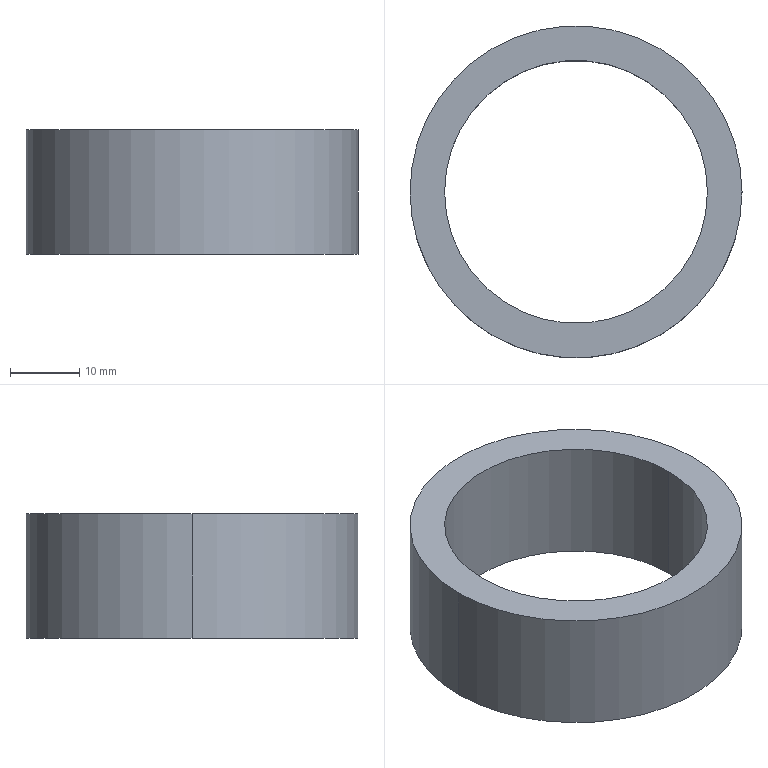Part | SolidWorks | features Extrusion 1 | 1 solid | 6 faces | box 48 x 48 x 18 mm | volume 12158 mm3 | cylinder 4 | plane 2 | commonest cylinder face diameters 38 x2 48 x2
STEP:
#1=CARTESIAN_POINT('',(-19.,0.,18.));
#2=VERTEX_POINT('',#1);
#3=CARTESIAN_POINT('',(19.,0.,18.));
#4=VERTEX_POINT('',#3);
#5=CARTESIAN_POINT('',(0.,0.,18.));
#6=DIRECTION('',(0.,0.,1.));
#7=DIRECTION('',(1.,0.,0.));
#8=AXIS2_PLACEMENT_3D('',#5,#6,#7);
#9=CIRCLE('',#8,19.);
#10=EDGE_CURVE('',#2,#4,#9,.T.);
#11=ORIENTED_EDGE('',*,*,#10,.T.);
#12=CARTESIAN_POINT('',(19.,0.,0.));
#13=VERTEX_POINT('',#12);
#14=CARTESIAN_POINT('',(19.,0.,18.));
#15=DIRECTION('',(0.,0.,-1.));
#16=VECTOR('',#15,1000.);
#17=LINE('',#14,#16);
#18=EDGE_CURVE('',#4,#13,#17,.T.);
#19=ORIENTED_EDGE('',*,*,#18,.T.);
#20=CARTESIAN_POINT('',(-19.,0.,0.));
#21=VERTEX_POINT('',#20);
#22=CARTESIAN_POINT('',(0.,0.,0.));
#23=DIRECTION('',(0.,0.,1.));
#24=DIRECTION('',(1.,0.,0.));
#25=AXIS2_PLACEMENT_3D('',#22,#23,#24);
#26=CIRCLE('',#25,19.);
#27=EDGE_CURVE('',#21,#13,#26,.T.);
#28=ORIENTED_EDGE('',*,*,#27,.F.);
#29=CARTESIAN_POINT('',(-19.,0.,18.));
#30=DIRECTION('',(0.,0.,-1.));
#31=VECTOR('',#30,1000.);
#32=LINE('',#29,#31);
#33=EDGE_CURVE('',#2,#21,#32,.T.);
#34=ORIENTED_EDGE('',*,*,#33,.F.);
#35=EDGE_LOOP('',(#11,#19,#28,#34));
#36=FACE_OUTER_BOUND('',#35,.T.);
#37=CARTESIAN_POINT('',(0.,0.,18.));
#38=DIRECTION('',(0.,0.,-1.));
#39=DIRECTION('',(-1.,0.,0.));
#40=AXIS2_PLACEMENT_3D('',#37,#38,#39);
#41=CYLINDRICAL_SURFACE('',#40,19.);
#42=ADVANCED_FACE('',(#36),#41,.F.);
#43=CARTESIAN_POINT('',(24.,0.,18.));
#44=VERTEX_POINT('',#43);
#45=CARTESIAN_POINT('',(-24.,0.,18.));
#46=VERTEX_POINT('',#45);
#47=CARTESIAN_POINT('',(0.,0.,18.));
#48=DIRECTION('',(0.,0.,1.));
#49=DIRECTION('',(1.,0.,0.));
#50=AXIS2_PLACEMENT_3D('',#47,#48,#49);
#51=CIRCLE('',#50,24.);
#52=EDGE_CURVE('',#44,#46,#51,.T.);
#53=ORIENTED_EDGE('',*,*,#52,.F.);
#54=CARTESIAN_POINT('',(24.,0.,0.));
#55=VERTEX_POINT('',#54);
#56=CARTESIAN_POINT('',(24.,0.,18.));
#57=DIRECTION('',(0.,0.,-1.));
#58=VECTOR('',#57,1000.);
#59=LINE('',#56,#58);
#60=EDGE_CURVE('',#44,#55,#59,.T.);
#61=ORIENTED_EDGE('',*,*,#60,.T.);
#62=CARTESIAN_POINT('',(-24.,0.,0.));
#63=VERTEX_POINT('',#62);
#64=CARTESIAN_POINT('',(0.,0.,0.));
#65=DIRECTION('',(0.,0.,1.));
#66=DIRECTION('',(1.,0.,0.));
#67=AXIS2_PLACEMENT_3D('',#64,#65,#66);
#68=CIRCLE('',#67,24.);
#69=EDGE_CURVE('',#55,#63,#68,.T.);
#70=ORIENTED_EDGE('',*,*,#69,.T.);
#71=CARTESIAN_POINT('',(-24.,0.,18.));
#72=DIRECTION('',(0.,0.,-1.));
#73=VECTOR('',#72,1000.);
#74=LINE('',#71,#73);
#75=EDGE_CURVE('',#46,#63,#74,.T.);
#76=ORIENTED_EDGE('',*,*,#75,.F.);
#77=EDGE_LOOP('',(#53,#61,#70,#76));
#78=FACE_OUTER_BOUND('',#77,.T.);
#79=CARTESIAN_POINT('',(0.,0.,18.));
#80=DIRECTION('',(0.,0.,-1.));
#81=DIRECTION('',(-1.,0.,0.));
#82=AXIS2_PLACEMENT_3D('',#79,#80,#81);
#83=CYLINDRICAL_SURFACE('',#82,24.);
#84=ADVANCED_FACE('',(#78),#83,.T.);
#85=CARTESIAN_POINT('',(0.,0.,18.));
#86=DIRECTION('',(0.,0.,1.));
#87=DIRECTION('',(1.,0.,0.));
#88=AXIS2_PLACEMENT_3D('',#85,#86,#87);
#89=CIRCLE('',#88,24.);
#90=EDGE_CURVE('',#46,#44,#89,.T.);
#91=ORIENTED_EDGE('',*,*,#90,.T.);
#92=ORIENTED_EDGE('',*,*,#52,.T.);
#93=EDGE_LOOP('',(#91,#92));
#94=FACE_OUTER_BOUND('',#93,.T.);
#95=ORIENTED_EDGE('',*,*,#10,.F.);
#96=CARTESIAN_POINT('',(0.,0.,18.));
#97=DIRECTION('',(0.,0.,1.));
#98=DIRECTION('',(1.,0.,0.));
#99=AXIS2_PLACEMENT_3D('',#96,#97,#98);
#100=CIRCLE('',#99,19.);
#101=EDGE_CURVE('',#4,#2,#100,.T.);
#102=ORIENTED_EDGE('',*,*,#101,.F.);
#103=EDGE_LOOP('',(#95,#102));
#104=FACE_BOUND('',#103,.T.);
#105=CARTESIAN_POINT('',(0.,0.,18.));
#106=DIRECTION('',(0.,0.,1.));
#107=DIRECTION('',(1.,0.,0.));
#108=AXIS2_PLACEMENT_3D('',#105,#106,#107);
#109=PLANE('',#108);
#110=ADVANCED_FACE('',(#94,#104),#109,.T.);
#111=CARTESIAN_POINT('',(0.,0.,0.));
#112=DIRECTION('',(0.,0.,1.));
#113=DIRECTION('',(1.,0.,0.));
#114=AXIS2_PLACEMENT_3D('',#111,#112,#113);
#115=CIRCLE('',#114,24.);
#116=EDGE_CURVE('',#63,#55,#115,.T.);
#117=ORIENTED_EDGE('',*,*,#116,.F.);
#118=ORIENTED_EDGE('',*,*,#69,.F.);
#119=EDGE_LOOP('',(#117,#118));
#120=FACE_OUTER_BOUND('',#119,.T.);
#121=ORIENTED_EDGE('',*,*,#27,.T.);
#122=CARTESIAN_POINT('',(0.,0.,0.));
#123=DIRECTION('',(0.,0.,1.));
#124=DIRECTION('',(1.,0.,0.));
#125=AXIS2_PLACEMENT_3D('',#122,#123,#124);
#126=CIRCLE('',#125,19.);
#127=EDGE_CURVE('',#13,#21,#126,.T.);
#128=ORIENTED_EDGE('',*,*,#127,.T.);
#129=EDGE_LOOP('',(#121,#128));
#130=FACE_BOUND('',#129,.T.);
#131=CARTESIAN_POINT('',(0.,0.,0.));
#132=DIRECTION('',(0.,0.,1.));
#133=DIRECTION('',(1.,0.,0.));
#134=AXIS2_PLACEMENT_3D('',#131,#132,#133);
#135=PLANE('',#134);
#136=ADVANCED_FACE('',(#120,#130),#135,.F.);
#137=ORIENTED_EDGE('',*,*,#60,.F.);
#138=ORIENTED_EDGE('',*,*,#90,.F.);
#139=ORIENTED_EDGE('',*,*,#75,.T.);
#140=ORIENTED_EDGE('',*,*,#116,.T.);
#141=EDGE_LOOP('',(#137,#138,#139,#140));
#142=FACE_OUTER_BOUND('',#141,.T.);
#143=CARTESIAN_POINT('',(0.,0.,18.));
#144=DIRECTION('',(0.,0.,-1.));
#145=DIRECTION('',(-1.,0.,0.));
#146=AXIS2_PLACEMENT_3D('',#143,#144,#145);
#147=CYLINDRICAL_SURFACE('',#146,24.);
#148=ADVANCED_FACE('',(#142),#147,.T.);
#149=ORIENTED_EDGE('',*,*,#18,.F.);
#150=ORIENTED_EDGE('',*,*,#101,.T.);
#151=ORIENTED_EDGE('',*,*,#33,.T.);
#152=ORIENTED_EDGE('',*,*,#127,.F.);
#153=EDGE_LOOP('',(#149,#150,#151,#152));
#154=FACE_OUTER_BOUND('',#153,.T.);
#155=CARTESIAN_POINT('',(0.,0.,18.));
#156=DIRECTION('',(0.,0.,-1.));
#157=DIRECTION('',(-1.,0.,0.));
#158=AXIS2_PLACEMENT_3D('',#155,#156,#157);
#159=CYLINDRICAL_SURFACE('',#158,19.);
#160=ADVANCED_FACE('',(#154),#159,.F.);
#161=CLOSED_SHELL('',(#42,#84,#110,#136,#148,#160));
#162=MANIFOLD_SOLID_BREP('',#161);
#163=CARTESIAN_POINT('',(0.,0.,0.));
#164=DIRECTION('',(0.,0.,1.));
#165=DIRECTION('',(1.,0.,0.));
#166=AXIS2_PLACEMENT_3D('',#163,#164,#165);
#167=(LENGTH_UNIT()NAMED_UNIT(*)SI_UNIT(.MILLI.,.METRE.));
#168=UNCERTAINTY_MEASURE_WITH_UNIT(LENGTH_MEASURE(0.00001),#167,'','');
#169=(NAMED_UNIT(*)PLANE_ANGLE_UNIT()SI_UNIT($,.RADIAN.));
#170=(NAMED_UNIT(*)SI_UNIT($,.STERADIAN.)SOLID_ANGLE_UNIT());
#171=(GEOMETRIC_REPRESENTATION_CONTEXT(3)GLOBAL_UNCERTAINTY_ASSIGNED_CONTEXT((#168))GLOBAL_UNIT_ASSIGNED_CONTEXT((#167,#169,#170))REPRESENTATION_CONTEXT('',''));
#172=ADVANCED_BREP_SHAPE_REPRESENTATION('',(#162,#166),#171);